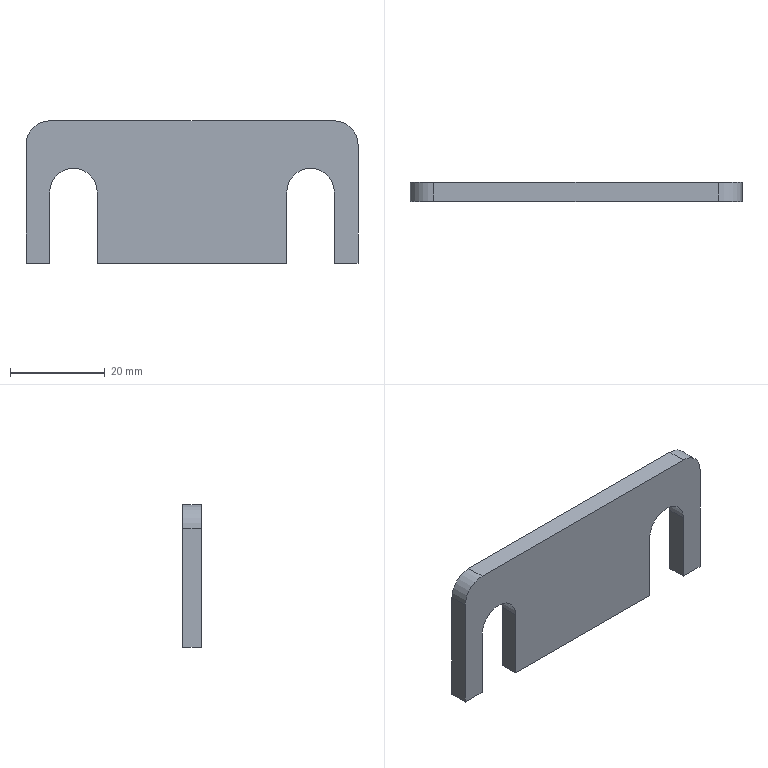Part | SolidWorks | features MirrorStock 1 | 1 solid | 18 faces | box 70 x 4 x 30 mm | volume 6843 mm3 | plane 12 | cylinder 6 | commonest cylinder face diameters 10 x6
STEP:
#1=CARTESIAN_POINT('',(20.,4.,15.));
#2=VERTEX_POINT('',#1);
#3=CARTESIAN_POINT('',(25.,4.,20.));
#4=VERTEX_POINT('',#3);
#5=CARTESIAN_POINT('',(25.,4.,15.));
#6=DIRECTION('',(0.,1.,0.));
#7=DIRECTION('',(0.,0.,1.));
#8=AXIS2_PLACEMENT_3D('',#5,#6,#7);
#9=CIRCLE('',#8,5.);
#10=EDGE_CURVE('',#2,#4,#9,.T.);
#11=ORIENTED_EDGE('',*,*,#10,.T.);
#12=CARTESIAN_POINT('',(25.,0.,20.));
#13=VERTEX_POINT('',#12);
#14=CARTESIAN_POINT('',(25.,4.,20.));
#15=DIRECTION('',(0.,-1.,0.));
#16=VECTOR('',#15,1000.);
#17=LINE('',#14,#16);
#18=EDGE_CURVE('',#4,#13,#17,.T.);
#19=ORIENTED_EDGE('',*,*,#18,.T.);
#20=CARTESIAN_POINT('',(20.,0.,15.));
#21=VERTEX_POINT('',#20);
#22=CARTESIAN_POINT('',(25.,0.,15.));
#23=DIRECTION('',(0.,1.,0.));
#24=DIRECTION('',(0.,0.,1.));
#25=AXIS2_PLACEMENT_3D('',#22,#23,#24);
#26=CIRCLE('',#25,5.);
#27=EDGE_CURVE('',#21,#13,#26,.T.);
#28=ORIENTED_EDGE('',*,*,#27,.F.);
#29=CARTESIAN_POINT('',(20.,4.,15.));
#30=DIRECTION('',(0.,-1.,0.));
#31=VECTOR('',#30,1000.);
#32=LINE('',#29,#31);
#33=EDGE_CURVE('',#2,#21,#32,.T.);
#34=ORIENTED_EDGE('',*,*,#33,.F.);
#35=EDGE_LOOP('',(#11,#19,#28,#34));
#36=FACE_OUTER_BOUND('',#35,.T.);
#37=CARTESIAN_POINT('',(25.,4.,15.));
#38=DIRECTION('',(0.,-1.,0.));
#39=DIRECTION('',(0.,0.,1.));
#40=AXIS2_PLACEMENT_3D('',#37,#38,#39);
#41=CYLINDRICAL_SURFACE('',#40,5.);
#42=ADVANCED_FACE('',(#36),#41,.F.);
#43=CARTESIAN_POINT('',(-30.,4.,15.));
#44=VERTEX_POINT('',#43);
#45=CARTESIAN_POINT('',(-25.,4.,20.));
#46=VERTEX_POINT('',#45);
#47=CARTESIAN_POINT('',(-25.,4.,15.));
#48=DIRECTION('',(0.,1.,0.));
#49=DIRECTION('',(0.,0.,-1.));
#50=AXIS2_PLACEMENT_3D('',#47,#48,#49);
#51=CIRCLE('',#50,5.);
#52=EDGE_CURVE('',#44,#46,#51,.T.);
#53=ORIENTED_EDGE('',*,*,#52,.T.);
#54=CARTESIAN_POINT('',(-25.,0.,20.));
#55=VERTEX_POINT('',#54);
#56=CARTESIAN_POINT('',(-25.,4.,20.));
#57=DIRECTION('',(0.,-1.,0.));
#58=VECTOR('',#57,1000.);
#59=LINE('',#56,#58);
#60=EDGE_CURVE('',#46,#55,#59,.T.);
#61=ORIENTED_EDGE('',*,*,#60,.T.);
#62=CARTESIAN_POINT('',(-30.,0.,15.));
#63=VERTEX_POINT('',#62);
#64=CARTESIAN_POINT('',(-25.,0.,15.));
#65=DIRECTION('',(0.,1.,0.));
#66=DIRECTION('',(0.,0.,-1.));
#67=AXIS2_PLACEMENT_3D('',#64,#65,#66);
#68=CIRCLE('',#67,5.);
#69=EDGE_CURVE('',#63,#55,#68,.T.);
#70=ORIENTED_EDGE('',*,*,#69,.F.);
#71=CARTESIAN_POINT('',(-30.,4.,15.));
#72=DIRECTION('',(0.,-1.,0.));
#73=VECTOR('',#72,1000.);
#74=LINE('',#71,#73);
#75=EDGE_CURVE('',#44,#63,#74,.T.);
#76=ORIENTED_EDGE('',*,*,#75,.F.);
#77=EDGE_LOOP('',(#53,#61,#70,#76));
#78=FACE_OUTER_BOUND('',#77,.T.);
#79=CARTESIAN_POINT('',(-25.,4.,15.));
#80=DIRECTION('',(0.,-1.,0.));
#81=DIRECTION('',(0.,0.,1.));
#82=AXIS2_PLACEMENT_3D('',#79,#80,#81);
#83=CYLINDRICAL_SURFACE('',#82,5.);
#84=ADVANCED_FACE('',(#78),#83,.F.);
#85=CARTESIAN_POINT('',(-30.,0.,0.));
#86=VERTEX_POINT('',#85);
#87=CARTESIAN_POINT('',(-30.,0.,0.));
#88=DIRECTION('',(0.,0.,1.));
#89=VECTOR('',#88,1000.);
#90=LINE('',#87,#89);
#91=EDGE_CURVE('',#86,#63,#90,.T.);
#92=ORIENTED_EDGE('',*,*,#91,.F.);
#93=CARTESIAN_POINT('',(-30.,4.,0.));
#94=VERTEX_POINT('',#93);
#95=CARTESIAN_POINT('',(-30.,4.,0.));
#96=DIRECTION('',(0.,-1.,0.));
#97=VECTOR('',#96,1000.);
#98=LINE('',#95,#97);
#99=EDGE_CURVE('',#94,#86,#98,.T.);
#100=ORIENTED_EDGE('',*,*,#99,.F.);
#101=CARTESIAN_POINT('',(-30.,4.,0.));
#102=DIRECTION('',(0.,0.,1.));
#103=VECTOR('',#102,1000.);
#104=LINE('',#101,#103);
#105=EDGE_CURVE('',#94,#44,#104,.T.);
#106=ORIENTED_EDGE('',*,*,#105,.T.);
#107=ORIENTED_EDGE('',*,*,#75,.T.);
#108=EDGE_LOOP('',(#92,#100,#106,#107));
#109=FACE_OUTER_BOUND('',#108,.T.);
#110=CARTESIAN_POINT('',(-30.,4.,0.));
#111=DIRECTION('',(-1.,0.,0.));
#112=DIRECTION('',(0.,0.,-1.));
#113=AXIS2_PLACEMENT_3D('',#110,#111,#112);
#114=PLANE('',#113);
#115=ADVANCED_FACE('',(#109),#114,.F.);
#116=ORIENTED_EDGE('',*,*,#60,.F.);
#117=CARTESIAN_POINT('',(-20.,4.,15.));
#118=VERTEX_POINT('',#117);
#119=CARTESIAN_POINT('',(-25.,4.,15.));
#120=DIRECTION('',(0.,1.,0.));
#121=DIRECTION('',(0.,0.,-1.));
#122=AXIS2_PLACEMENT_3D('',#119,#120,#121);
#123=CIRCLE('',#122,5.);
#124=EDGE_CURVE('',#46,#118,#123,.T.);
#125=ORIENTED_EDGE('',*,*,#124,.T.);
#126=CARTESIAN_POINT('',(-20.,0.,15.));
#127=VERTEX_POINT('',#126);
#128=CARTESIAN_POINT('',(-20.,4.,15.));
#129=DIRECTION('',(0.,-1.,0.));
#130=VECTOR('',#129,1000.);
#131=LINE('',#128,#130);
#132=EDGE_CURVE('',#118,#127,#131,.T.);
#133=ORIENTED_EDGE('',*,*,#132,.T.);
#134=CARTESIAN_POINT('',(-25.,0.,15.));
#135=DIRECTION('',(0.,1.,0.));
#136=DIRECTION('',(0.,0.,-1.));
#137=AXIS2_PLACEMENT_3D('',#134,#135,#136);
#138=CIRCLE('',#137,5.);
#139=EDGE_CURVE('',#55,#127,#138,.T.);
#140=ORIENTED_EDGE('',*,*,#139,.F.);
#141=EDGE_LOOP('',(#116,#125,#133,#140));
#142=FACE_OUTER_BOUND('',#141,.T.);
#143=CARTESIAN_POINT('',(-25.,4.,15.));
#144=DIRECTION('',(0.,-1.,0.));
#145=DIRECTION('',(0.,0.,1.));
#146=AXIS2_PLACEMENT_3D('',#143,#144,#145);
#147=CYLINDRICAL_SURFACE('',#146,5.);
#148=ADVANCED_FACE('',(#142),#147,.F.);
#149=CARTESIAN_POINT('',(-20.,0.,0.));
#150=VERTEX_POINT('',#149);
#151=CARTESIAN_POINT('',(-20.,0.,15.));
#152=DIRECTION('',(0.,0.,-1.));
#153=VECTOR('',#152,1000.);
#154=LINE('',#151,#153);
#155=EDGE_CURVE('',#127,#150,#154,.T.);
#156=ORIENTED_EDGE('',*,*,#155,.F.);
#157=ORIENTED_EDGE('',*,*,#132,.F.);
#158=CARTESIAN_POINT('',(-20.,4.,0.));
#159=VERTEX_POINT('',#158);
#160=CARTESIAN_POINT('',(-20.,4.,15.));
#161=DIRECTION('',(0.,0.,-1.));
#162=VECTOR('',#161,1000.);
#163=LINE('',#160,#162);
#164=EDGE_CURVE('',#118,#159,#163,.T.);
#165=ORIENTED_EDGE('',*,*,#164,.T.);
#166=CARTESIAN_POINT('',(-20.,4.,0.));
#167=DIRECTION('',(0.,-1.,0.));
#168=VECTOR('',#167,1000.);
#169=LINE('',#166,#168);
#170=EDGE_CURVE('',#159,#150,#169,.T.);
#171=ORIENTED_EDGE('',*,*,#170,.T.);
#172=EDGE_LOOP('',(#156,#157,#165,#171));
#173=FACE_OUTER_BOUND('',#172,.T.);
#174=CARTESIAN_POINT('',(-20.,4.,15.));
#175=DIRECTION('',(1.,0.,0.));
#176=DIRECTION('',(0.,0.,1.));
#177=AXIS2_PLACEMENT_3D('',#174,#175,#176);
#178=PLANE('',#177);
#179=ADVANCED_FACE('',(#173),#178,.F.);
#180=CARTESIAN_POINT('',(20.,0.,0.));
#181=VERTEX_POINT('',#180);
#182=CARTESIAN_POINT('',(-20.,0.,0.));
#183=DIRECTION('',(1.,0.,0.));
#184=VECTOR('',#183,1000.);
#185=LINE('',#182,#184);
#186=EDGE_CURVE('',#150,#181,#185,.T.);
#187=ORIENTED_EDGE('',*,*,#186,.F.);
#188=ORIENTED_EDGE('',*,*,#170,.F.);
#189=CARTESIAN_POINT('',(20.,4.,0.));
#190=VERTEX_POINT('',#189);
#191=CARTESIAN_POINT('',(-20.,4.,0.));
#192=DIRECTION('',(1.,0.,0.));
#193=VECTOR('',#192,1000.);
#194=LINE('',#191,#193);
#195=EDGE_CURVE('',#159,#190,#194,.T.);
#196=ORIENTED_EDGE('',*,*,#195,.T.);
#197=CARTESIAN_POINT('',(20.,4.,0.));
#198=DIRECTION('',(0.,-1.,0.));
#199=VECTOR('',#198,1000.);
#200=LINE('',#197,#199);
#201=EDGE_CURVE('',#190,#181,#200,.T.);
#202=ORIENTED_EDGE('',*,*,#201,.T.);
#203=EDGE_LOOP('',(#187,#188,#196,#202));
#204=FACE_OUTER_BOUND('',#203,.T.);
#205=CARTESIAN_POINT('',(-20.,4.,0.));
#206=DIRECTION('',(0.,0.,1.));
#207=DIRECTION('',(-1.,0.,0.));
#208=AXIS2_PLACEMENT_3D('',#205,#206,#207);
#209=PLANE('',#208);
#210=ADVANCED_FACE('',(#204),#209,.F.);
#211=CARTESIAN_POINT('',(20.,0.,15.));
#212=DIRECTION('',(0.,0.,1.));
#213=VECTOR('',#212,1000.);
#214=LINE('',#211,#213);
#215=EDGE_CURVE('',#181,#21,#214,.T.);
#216=ORIENTED_EDGE('',*,*,#215,.F.);
#217=ORIENTED_EDGE('',*,*,#201,.F.);
#218=CARTESIAN_POINT('',(20.,4.,15.));
#219=DIRECTION('',(0.,0.,1.));
#220=VECTOR('',#219,1000.);
#221=LINE('',#218,#220);
#222=EDGE_CURVE('',#190,#2,#221,.T.);
#223=ORIENTED_EDGE('',*,*,#222,.T.);
#224=ORIENTED_EDGE('',*,*,#33,.T.);
#225=EDGE_LOOP('',(#216,#217,#223,#224));
#226=FACE_OUTER_BOUND('',#225,.T.);
#227=CARTESIAN_POINT('',(20.,4.,15.));
#228=DIRECTION('',(-1.,0.,0.));
#229=DIRECTION('',(0.,0.,-1.));
#230=AXIS2_PLACEMENT_3D('',#227,#228,#229);
#231=PLANE('',#230);
#232=ADVANCED_FACE('',(#226),#231,.F.);
#233=ORIENTED_EDGE('',*,*,#18,.F.);
#234=CARTESIAN_POINT('',(30.,4.,15.));
#235=VERTEX_POINT('',#234);
#236=CARTESIAN_POINT('',(25.,4.,15.));
#237=DIRECTION('',(0.,1.,0.));
#238=DIRECTION('',(0.,0.,1.));
#239=AXIS2_PLACEMENT_3D('',#236,#237,#238);
#240=CIRCLE('',#239,5.);
#241=EDGE_CURVE('',#4,#235,#240,.T.);
#242=ORIENTED_EDGE('',*,*,#241,.T.);
#243=CARTESIAN_POINT('',(30.,0.,15.));
#244=VERTEX_POINT('',#243);
#245=CARTESIAN_POINT('',(30.,4.,15.));
#246=DIRECTION('',(0.,-1.,0.));
#247=VECTOR('',#246,1000.);
#248=LINE('',#245,#247);
#249=EDGE_CURVE('',#235,#244,#248,.T.);
#250=ORIENTED_EDGE('',*,*,#249,.T.);
#251=CARTESIAN_POINT('',(25.,0.,15.));
#252=DIRECTION('',(0.,1.,0.));
#253=DIRECTION('',(0.,0.,1.));
#254=AXIS2_PLACEMENT_3D('',#251,#252,#253);
#255=CIRCLE('',#254,5.);
#256=EDGE_CURVE('',#13,#244,#255,.T.);
#257=ORIENTED_EDGE('',*,*,#256,.F.);
#258=EDGE_LOOP('',(#233,#242,#250,#257));
#259=FACE_OUTER_BOUND('',#258,.T.);
#260=CARTESIAN_POINT('',(25.,4.,15.));
#261=DIRECTION('',(0.,-1.,0.));
#262=DIRECTION('',(0.,0.,1.));
#263=AXIS2_PLACEMENT_3D('',#260,#261,#262);
#264=CYLINDRICAL_SURFACE('',#263,5.);
#265=ADVANCED_FACE('',(#259),#264,.F.);
#266=CARTESIAN_POINT('',(30.,0.,0.));
#267=VERTEX_POINT('',#266);
#268=CARTESIAN_POINT('',(30.,0.,0.));
#269=DIRECTION('',(0.,0.,-1.));
#270=VECTOR('',#269,1000.);
#271=LINE('',#268,#270);
#272=EDGE_CURVE('',#244,#267,#271,.T.);
#273=ORIENTED_EDGE('',*,*,#272,.F.);
#274=ORIENTED_EDGE('',*,*,#249,.F.);
#275=CARTESIAN_POINT('',(30.,4.,0.));
#276=VERTEX_POINT('',#275);
#277=CARTESIAN_POINT('',(30.,4.,0.));
#278=DIRECTION('',(0.,0.,-1.));
#279=VECTOR('',#278,1000.);
#280=LINE('',#277,#279);
#281=EDGE_CURVE('',#235,#276,#280,.T.);
#282=ORIENTED_EDGE('',*,*,#281,.T.);
#283=CARTESIAN_POINT('',(30.,4.,0.));
#284=DIRECTION('',(0.,-1.,0.));
#285=VECTOR('',#284,1000.);
#286=LINE('',#283,#285);
#287=EDGE_CURVE('',#276,#267,#286,.T.);
#288=ORIENTED_EDGE('',*,*,#287,.T.);
#289=EDGE_LOOP('',(#273,#274,#282,#288));
#290=FACE_OUTER_BOUND('',#289,.T.);
#291=CARTESIAN_POINT('',(30.,4.,0.));
#292=DIRECTION('',(1.,0.,0.));
#293=DIRECTION('',(0.,0.,1.));
#294=AXIS2_PLACEMENT_3D('',#291,#292,#293);
#295=PLANE('',#294);
#296=ADVANCED_FACE('',(#290),#295,.F.);
#297=CARTESIAN_POINT('',(35.,0.,0.));
#298=VERTEX_POINT('',#297);
#299=CARTESIAN_POINT('',(35.,0.,0.));
#300=DIRECTION('',(1.,0.,0.));
#301=VECTOR('',#300,1000.);
#302=LINE('',#299,#301);
#303=EDGE_CURVE('',#267,#298,#302,.T.);
#304=ORIENTED_EDGE('',*,*,#303,.F.);
#305=ORIENTED_EDGE('',*,*,#287,.F.);
#306=CARTESIAN_POINT('',(35.,4.,0.));
#307=VERTEX_POINT('',#306);
#308=CARTESIAN_POINT('',(35.,4.,0.));
#309=DIRECTION('',(1.,0.,0.));
#310=VECTOR('',#309,1000.);
#311=LINE('',#308,#310);
#312=EDGE_CURVE('',#276,#307,#311,.T.);
#313=ORIENTED_EDGE('',*,*,#312,.T.);
#314=CARTESIAN_POINT('',(35.,4.,0.));
#315=DIRECTION('',(0.,-1.,0.));
#316=VECTOR('',#315,1000.);
#317=LINE('',#314,#316);
#318=EDGE_CURVE('',#307,#298,#317,.T.);
#319=ORIENTED_EDGE('',*,*,#318,.T.);
#320=EDGE_LOOP('',(#304,#305,#313,#319));
#321=FACE_OUTER_BOUND('',#320,.T.);
#322=CARTESIAN_POINT('',(35.,4.,0.));
#323=DIRECTION('',(0.,0.,1.));
#324=DIRECTION('',(-1.,0.,0.));
#325=AXIS2_PLACEMENT_3D('',#322,#323,#324);
#326=PLANE('',#325);
#327=ADVANCED_FACE('',(#321),#326,.F.);
#328=CARTESIAN_POINT('',(35.,0.,25.));
#329=VERTEX_POINT('',#328);
#330=CARTESIAN_POINT('',(35.,0.,25.));
#331=DIRECTION('',(0.,0.,1.));
#332=VECTOR('',#331,1000.);
#333=LINE('',#330,#332);
#334=EDGE_CURVE('',#298,#329,#333,.T.);
#335=ORIENTED_EDGE('',*,*,#334,.F.);
#336=ORIENTED_EDGE('',*,*,#318,.F.);
#337=CARTESIAN_POINT('',(35.,4.,25.));
#338=VERTEX_POINT('',#337);
#339=CARTESIAN_POINT('',(35.,4.,25.));
#340=DIRECTION('',(0.,0.,1.));
#341=VECTOR('',#340,1000.);
#342=LINE('',#339,#341);
#343=EDGE_CURVE('',#307,#338,#342,.T.);
#344=ORIENTED_EDGE('',*,*,#343,.T.);
#345=CARTESIAN_POINT('',(35.,4.,25.));
#346=DIRECTION('',(0.,-1.,0.));
#347=VECTOR('',#346,1000.);
#348=LINE('',#345,#347);
#349=EDGE_CURVE('',#338,#329,#348,.T.);
#350=ORIENTED_EDGE('',*,*,#349,.T.);
#351=EDGE_LOOP('',(#335,#336,#344,#350));
#352=FACE_OUTER_BOUND('',#351,.T.);
#353=CARTESIAN_POINT('',(35.,4.,25.));
#354=DIRECTION('',(-1.,0.,0.));
#355=DIRECTION('',(0.,0.,-1.));
#356=AXIS2_PLACEMENT_3D('',#353,#354,#355);
#357=PLANE('',#356);
#358=ADVANCED_FACE('',(#352),#357,.F.);
#359=CARTESIAN_POINT('',(30.,0.,30.));
#360=VERTEX_POINT('',#359);
#361=CARTESIAN_POINT('',(30.,0.,25.));
#362=DIRECTION('',(0.,-1.,0.));
#363=DIRECTION('',(0.,0.,1.));
#364=AXIS2_PLACEMENT_3D('',#361,#362,#363);
#365=CIRCLE('',#364,5.);
#366=EDGE_CURVE('',#329,#360,#365,.T.);
#367=ORIENTED_EDGE('',*,*,#366,.F.);
#368=ORIENTED_EDGE('',*,*,#349,.F.);
#369=CARTESIAN_POINT('',(30.,4.,30.));
#370=VERTEX_POINT('',#369);
#371=CARTESIAN_POINT('',(30.,4.,25.));
#372=DIRECTION('',(0.,-1.,0.));
#373=DIRECTION('',(0.,0.,1.));
#374=AXIS2_PLACEMENT_3D('',#371,#372,#373);
#375=CIRCLE('',#374,5.);
#376=EDGE_CURVE('',#338,#370,#375,.T.);
#377=ORIENTED_EDGE('',*,*,#376,.T.);
#378=CARTESIAN_POINT('',(30.,4.,30.));
#379=DIRECTION('',(0.,-1.,0.));
#380=VECTOR('',#379,1000.);
#381=LINE('',#378,#380);
#382=EDGE_CURVE('',#370,#360,#381,.T.);
#383=ORIENTED_EDGE('',*,*,#382,.T.);
#384=EDGE_LOOP('',(#367,#368,#377,#383));
#385=FACE_OUTER_BOUND('',#384,.T.);
#386=CARTESIAN_POINT('',(30.,4.,25.));
#387=DIRECTION('',(0.,-1.,0.));
#388=DIRECTION('',(0.,0.,1.));
#389=AXIS2_PLACEMENT_3D('',#386,#387,#388);
#390=CYLINDRICAL_SURFACE('',#389,5.);
#391=ADVANCED_FACE('',(#385),#390,.T.);
#392=CARTESIAN_POINT('',(-30.,0.,30.));
#393=VERTEX_POINT('',#392);
#394=CARTESIAN_POINT('',(30.,0.,30.));
#395=DIRECTION('',(-1.,0.,0.));
#396=VECTOR('',#395,1000.);
#397=LINE('',#394,#396);
#398=EDGE_CURVE('',#360,#393,#397,.T.);
#399=ORIENTED_EDGE('',*,*,#398,.F.);
#400=ORIENTED_EDGE('',*,*,#382,.F.);
#401=CARTESIAN_POINT('',(-30.,4.,30.));
#402=VERTEX_POINT('',#401);
#403=CARTESIAN_POINT('',(30.,4.,30.));
#404=DIRECTION('',(-1.,0.,0.));
#405=VECTOR('',#404,1000.);
#406=LINE('',#403,#405);
#407=EDGE_CURVE('',#370,#402,#406,.T.);
#408=ORIENTED_EDGE('',*,*,#407,.T.);
#409=CARTESIAN_POINT('',(-30.,4.,30.));
#410=DIRECTION('',(0.,-1.,0.));
#411=VECTOR('',#410,1000.);
#412=LINE('',#409,#411);
#413=EDGE_CURVE('',#402,#393,#412,.T.);
#414=ORIENTED_EDGE('',*,*,#413,.T.);
#415=EDGE_LOOP('',(#399,#400,#408,#414));
#416=FACE_OUTER_BOUND('',#415,.T.);
#417=CARTESIAN_POINT('',(30.,4.,30.));
#418=DIRECTION('',(0.,0.,-1.));
#419=DIRECTION('',(1.,0.,0.));
#420=AXIS2_PLACEMENT_3D('',#417,#418,#419);
#421=PLANE('',#420);
#422=ADVANCED_FACE('',(#416),#421,.F.);
#423=CARTESIAN_POINT('',(-35.,0.,25.));
#424=VERTEX_POINT('',#423);
#425=CARTESIAN_POINT('',(-30.,0.,25.));
#426=DIRECTION('',(0.,-1.,0.));
#427=DIRECTION('',(0.,0.,-1.));
#428=AXIS2_PLACEMENT_3D('',#425,#426,#427);
#429=CIRCLE('',#428,5.);
#430=EDGE_CURVE('',#393,#424,#429,.T.);
#431=ORIENTED_EDGE('',*,*,#430,.F.);
#432=ORIENTED_EDGE('',*,*,#413,.F.);
#433=CARTESIAN_POINT('',(-35.,4.,25.));
#434=VERTEX_POINT('',#433);
#435=CARTESIAN_POINT('',(-30.,4.,25.));
#436=DIRECTION('',(0.,-1.,0.));
#437=DIRECTION('',(0.,0.,-1.));
#438=AXIS2_PLACEMENT_3D('',#435,#436,#437);
#439=CIRCLE('',#438,5.);
#440=EDGE_CURVE('',#402,#434,#439,.T.);
#441=ORIENTED_EDGE('',*,*,#440,.T.);
#442=CARTESIAN_POINT('',(-35.,4.,25.));
#443=DIRECTION('',(0.,-1.,0.));
#444=VECTOR('',#443,1000.);
#445=LINE('',#442,#444);
#446=EDGE_CURVE('',#434,#424,#445,.T.);
#447=ORIENTED_EDGE('',*,*,#446,.T.);
#448=EDGE_LOOP('',(#431,#432,#441,#447));
#449=FACE_OUTER_BOUND('',#448,.T.);
#450=CARTESIAN_POINT('',(-30.,4.,25.));
#451=DIRECTION('',(0.,-1.,0.));
#452=DIRECTION('',(0.,0.,1.));
#453=AXIS2_PLACEMENT_3D('',#450,#451,#452);
#454=CYLINDRICAL_SURFACE('',#453,5.);
#455=ADVANCED_FACE('',(#449),#454,.T.);
#456=CARTESIAN_POINT('',(-35.,0.,0.));
#457=VERTEX_POINT('',#456);
#458=CARTESIAN_POINT('',(-35.,0.,25.));
#459=DIRECTION('',(0.,0.,-1.));
#460=VECTOR('',#459,1000.);
#461=LINE('',#458,#460);
#462=EDGE_CURVE('',#424,#457,#461,.T.);
#463=ORIENTED_EDGE('',*,*,#462,.F.);
#464=ORIENTED_EDGE('',*,*,#446,.F.);
#465=CARTESIAN_POINT('',(-35.,4.,0.));
#466=VERTEX_POINT('',#465);
#467=CARTESIAN_POINT('',(-35.,4.,25.));
#468=DIRECTION('',(0.,0.,-1.));
#469=VECTOR('',#468,1000.);
#470=LINE('',#467,#469);
#471=EDGE_CURVE('',#434,#466,#470,.T.);
#472=ORIENTED_EDGE('',*,*,#471,.T.);
#473=CARTESIAN_POINT('',(-35.,4.,0.));
#474=DIRECTION('',(0.,-1.,0.));
#475=VECTOR('',#474,1000.);
#476=LINE('',#473,#475);
#477=EDGE_CURVE('',#466,#457,#476,.T.);
#478=ORIENTED_EDGE('',*,*,#477,.T.);
#479=EDGE_LOOP('',(#463,#464,#472,#478));
#480=FACE_OUTER_BOUND('',#479,.T.);
#481=CARTESIAN_POINT('',(-35.,4.,25.));
#482=DIRECTION('',(1.,0.,0.));
#483=DIRECTION('',(0.,0.,1.));
#484=AXIS2_PLACEMENT_3D('',#481,#482,#483);
#485=PLANE('',#484);
#486=ADVANCED_FACE('',(#480),#485,.F.);
#487=CARTESIAN_POINT('',(-35.,0.,0.));
#488=DIRECTION('',(1.,0.,0.));
#489=VECTOR('',#488,1000.);
#490=LINE('',#487,#489);
#491=EDGE_CURVE('',#457,#86,#490,.T.);
#492=ORIENTED_EDGE('',*,*,#491,.F.);
#493=ORIENTED_EDGE('',*,*,#477,.F.);
#494=CARTESIAN_POINT('',(-35.,4.,0.));
#495=DIRECTION('',(1.,0.,0.));
#496=VECTOR('',#495,1000.);
#497=LINE('',#494,#496);
#498=EDGE_CURVE('',#466,#94,#497,.T.);
#499=ORIENTED_EDGE('',*,*,#498,.T.);
#500=ORIENTED_EDGE('',*,*,#99,.T.);
#501=EDGE_LOOP('',(#492,#493,#499,#500));
#502=FACE_OUTER_BOUND('',#501,.T.);
#503=CARTESIAN_POINT('',(-35.,4.,0.));
#504=DIRECTION('',(0.,0.,1.));
#505=DIRECTION('',(-1.,0.,0.));
#506=AXIS2_PLACEMENT_3D('',#503,#504,#505);
#507=PLANE('',#506);
#508=ADVANCED_FACE('',(#502),#507,.F.);
#509=ORIENTED_EDGE('',*,*,#105,.F.);
#510=ORIENTED_EDGE('',*,*,#498,.F.);
#511=ORIENTED_EDGE('',*,*,#471,.F.);
#512=ORIENTED_EDGE('',*,*,#440,.F.);
#513=ORIENTED_EDGE('',*,*,#407,.F.);
#514=ORIENTED_EDGE('',*,*,#376,.F.);
#515=ORIENTED_EDGE('',*,*,#343,.F.);
#516=ORIENTED_EDGE('',*,*,#312,.F.);
#517=ORIENTED_EDGE('',*,*,#281,.F.);
#518=ORIENTED_EDGE('',*,*,#241,.F.);
#519=ORIENTED_EDGE('',*,*,#10,.F.);
#520=ORIENTED_EDGE('',*,*,#222,.F.);
#521=ORIENTED_EDGE('',*,*,#195,.F.);
#522=ORIENTED_EDGE('',*,*,#164,.F.);
#523=ORIENTED_EDGE('',*,*,#124,.F.);
#524=ORIENTED_EDGE('',*,*,#52,.F.);
#525=EDGE_LOOP('',(#509,#510,#511,#512,#513,#514,#515,#516,#517,#518,#519,#520,#521,#522,#523,#524));
#526=FACE_OUTER_BOUND('',#525,.T.);
#527=CARTESIAN_POINT('',(-25.,4.,15.));
#528=DIRECTION('',(0.,1.,0.));
#529=DIRECTION('',(0.,0.,-1.));
#530=AXIS2_PLACEMENT_3D('',#527,#528,#529);
#531=PLANE('',#530);
#532=ADVANCED_FACE('',(#526),#531,.T.);
#533=ORIENTED_EDGE('',*,*,#91,.T.);
#534=ORIENTED_EDGE('',*,*,#69,.T.);
#535=ORIENTED_EDGE('',*,*,#139,.T.);
#536=ORIENTED_EDGE('',*,*,#155,.T.);
#537=ORIENTED_EDGE('',*,*,#186,.T.);
#538=ORIENTED_EDGE('',*,*,#215,.T.);
#539=ORIENTED_EDGE('',*,*,#27,.T.);
#540=ORIENTED_EDGE('',*,*,#256,.T.);
#541=ORIENTED_EDGE('',*,*,#272,.T.);
#542=ORIENTED_EDGE('',*,*,#303,.T.);
#543=ORIENTED_EDGE('',*,*,#334,.T.);
#544=ORIENTED_EDGE('',*,*,#366,.T.);
#545=ORIENTED_EDGE('',*,*,#398,.T.);
#546=ORIENTED_EDGE('',*,*,#430,.T.);
#547=ORIENTED_EDGE('',*,*,#462,.T.);
#548=ORIENTED_EDGE('',*,*,#491,.T.);
#549=EDGE_LOOP('',(#533,#534,#535,#536,#537,#538,#539,#540,#541,#542,#543,#544,#545,#546,#547,#548));
#550=FACE_OUTER_BOUND('',#549,.T.);
#551=CARTESIAN_POINT('',(-25.,0.,15.));
#552=DIRECTION('',(0.,1.,0.));
#553=DIRECTION('',(0.,0.,-1.));
#554=AXIS2_PLACEMENT_3D('',#551,#552,#553);
#555=PLANE('',#554);
#556=ADVANCED_FACE('',(#550),#555,.F.);
#557=CLOSED_SHELL('',(#42,#84,#115,#148,#179,#210,#232,#265,#296,#327,#358,#391,#422,#455,#486,#508,#532,#556));
#558=MANIFOLD_SOLID_BREP('',#557);
#559=CARTESIAN_POINT('',(0.,0.,0.));
#560=DIRECTION('',(0.,0.,1.));
#561=DIRECTION('',(1.,0.,0.));
#562=AXIS2_PLACEMENT_3D('',#559,#560,#561);
#563=(LENGTH_UNIT()NAMED_UNIT(*)SI_UNIT(.MILLI.,.METRE.));
#564=UNCERTAINTY_MEASURE_WITH_UNIT(LENGTH_MEASURE(0.00001),#563,'','');
#565=(NAMED_UNIT(*)PLANE_ANGLE_UNIT()SI_UNIT($,.RADIAN.));
#566=(NAMED_UNIT(*)SI_UNIT($,.STERADIAN.)SOLID_ANGLE_UNIT());
#567=(GEOMETRIC_REPRESENTATION_CONTEXT(3)GLOBAL_UNCERTAINTY_ASSIGNED_CONTEXT((#564))GLOBAL_UNIT_ASSIGNED_CONTEXT((#563,#565,#566))REPRESENTATION_CONTEXT('',''));
#568=ADVANCED_BREP_SHAPE_REPRESENTATION('',(#558,#562),#567);